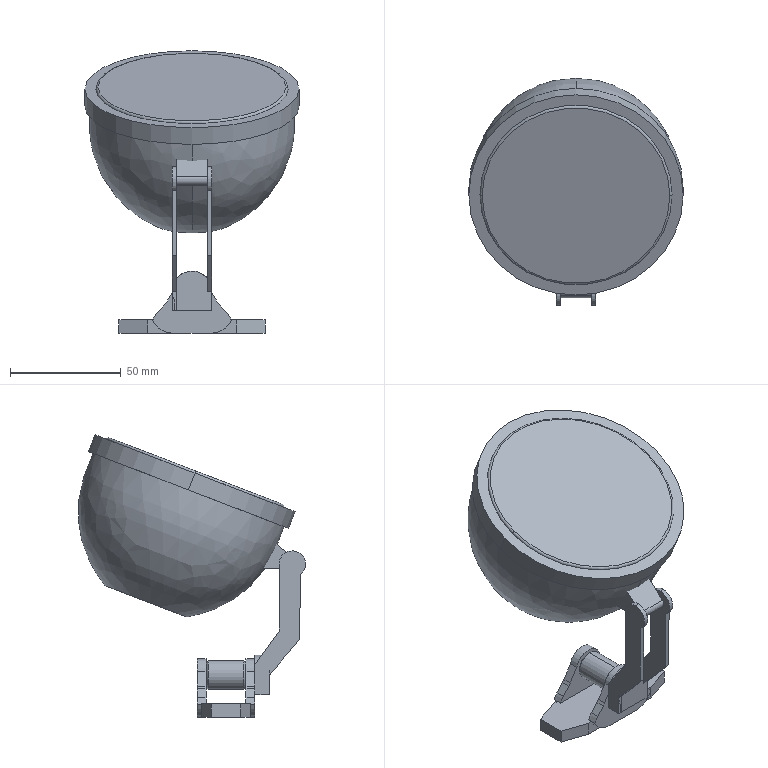Part | STEP file | ZAROWKA_MALA_01V11 | 10 solids | 121 faces | box 96.622 x 102.595 x 127.367 mm | volume 131229 mm3 | plane 67 | cylinder 34 | cone 12 | spline 4 | other 2 | torus 2 | commonest cylinder face diameters 20 x12 12 x4 86.622 x4 18 x3 4 x2 13 x2